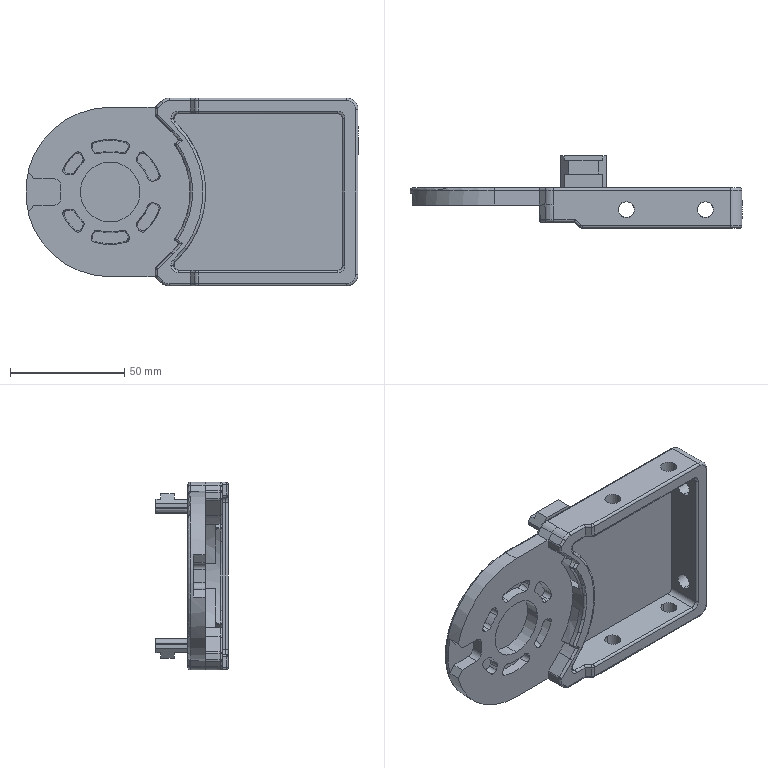Part | SolidWorks | features ICE 3, BaseBody 1 | 1 solid | 333 faces | box 145.118 x 31.5 x 82 mm | volume 67988 mm3 | cylinder 131 | plane 114 | cone 57 | torus 20 | spline 7 | sphere 4 | commonest cylinder face diameters 3.2 x36 4 x34 2 x33 7 x12 4.4 x6 10 x6